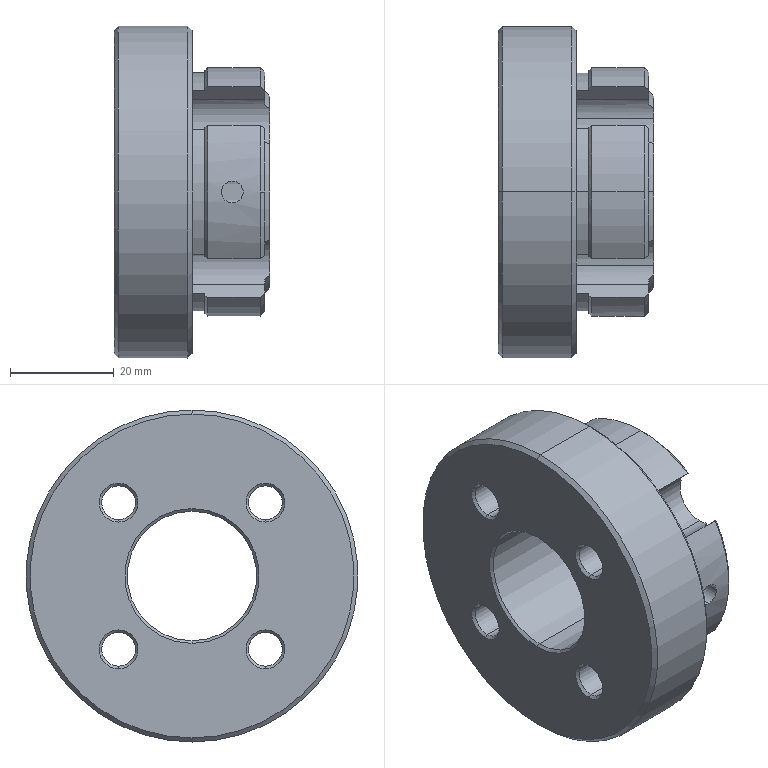Part | SolidWorks | features BaseBody 1 | 1 solid | 85 faces | box 30 x 64 x 64 mm | volume 51096 mm3 | cylinder 32 | cone 30 | plane 23 | commonest cylinder face diameters 6.5 x8 10.5 x8 46 x5 48 x5 4.2 x2 25 x2